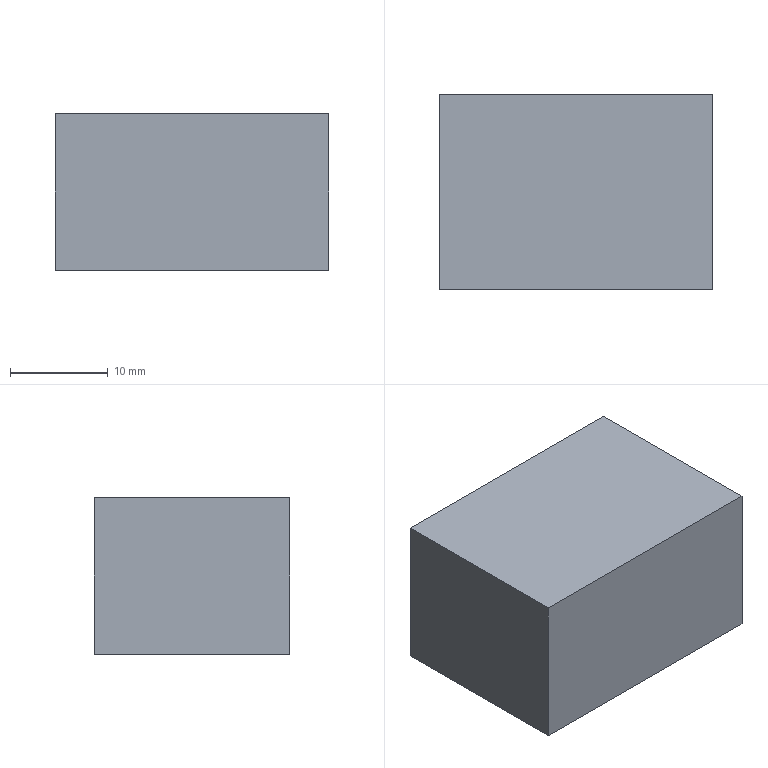Part | SolidWorks | features Extrusion 1 | 1 solid | 6 faces | box 28 x 20 x 16 mm | volume 8960 mm3 | plane 6
STEP:
#1=CARTESIAN_POINT('',(-14.,10.,8.));
#2=VERTEX_POINT('',#1);
#3=CARTESIAN_POINT('',(-14.,-10.,8.));
#4=VERTEX_POINT('',#3);
#5=CARTESIAN_POINT('',(-14.,10.,8.));
#6=DIRECTION('',(0.,-1.,0.));
#7=VECTOR('',#6,1000.);
#8=LINE('',#5,#7);
#9=EDGE_CURVE('',#2,#4,#8,.T.);
#10=ORIENTED_EDGE('',*,*,#9,.F.);
#11=CARTESIAN_POINT('',(-14.,10.,-8.));
#12=VERTEX_POINT('',#11);
#13=CARTESIAN_POINT('',(-14.,10.,-8.));
#14=DIRECTION('',(0.,0.,1.));
#15=VECTOR('',#14,1000.);
#16=LINE('',#13,#15);
#17=EDGE_CURVE('',#12,#2,#16,.T.);
#18=ORIENTED_EDGE('',*,*,#17,.F.);
#19=CARTESIAN_POINT('',(-14.,-10.,-8.));
#20=VERTEX_POINT('',#19);
#21=CARTESIAN_POINT('',(-14.,10.,-8.));
#22=DIRECTION('',(0.,-1.,0.));
#23=VECTOR('',#22,1000.);
#24=LINE('',#21,#23);
#25=EDGE_CURVE('',#12,#20,#24,.T.);
#26=ORIENTED_EDGE('',*,*,#25,.T.);
#27=CARTESIAN_POINT('',(-14.,-10.,-8.));
#28=DIRECTION('',(0.,0.,1.));
#29=VECTOR('',#28,1000.);
#30=LINE('',#27,#29);
#31=EDGE_CURVE('',#20,#4,#30,.T.);
#32=ORIENTED_EDGE('',*,*,#31,.T.);
#33=EDGE_LOOP('',(#10,#18,#26,#32));
#34=FACE_OUTER_BOUND('',#33,.T.);
#35=CARTESIAN_POINT('',(-14.,10.,-8.));
#36=DIRECTION('',(-1.,0.,0.));
#37=DIRECTION('',(0.,0.,1.));
#38=AXIS2_PLACEMENT_3D('',#35,#36,#37);
#39=PLANE('',#38);
#40=ADVANCED_FACE('',(#34),#39,.T.);
#41=CARTESIAN_POINT('',(14.,10.,8.));
#42=VERTEX_POINT('',#41);
#43=CARTESIAN_POINT('',(14.,10.,8.));
#44=DIRECTION('',(-1.,0.,0.));
#45=VECTOR('',#44,1000.);
#46=LINE('',#43,#45);
#47=EDGE_CURVE('',#42,#2,#46,.T.);
#48=ORIENTED_EDGE('',*,*,#47,.F.);
#49=CARTESIAN_POINT('',(14.,10.,-8.));
#50=VERTEX_POINT('',#49);
#51=CARTESIAN_POINT('',(14.,10.,-8.));
#52=DIRECTION('',(0.,0.,1.));
#53=VECTOR('',#52,1000.);
#54=LINE('',#51,#53);
#55=EDGE_CURVE('',#50,#42,#54,.T.);
#56=ORIENTED_EDGE('',*,*,#55,.F.);
#57=CARTESIAN_POINT('',(14.,10.,-8.));
#58=DIRECTION('',(-1.,0.,0.));
#59=VECTOR('',#58,1000.);
#60=LINE('',#57,#59);
#61=EDGE_CURVE('',#50,#12,#60,.T.);
#62=ORIENTED_EDGE('',*,*,#61,.T.);
#63=ORIENTED_EDGE('',*,*,#17,.T.);
#64=EDGE_LOOP('',(#48,#56,#62,#63));
#65=FACE_OUTER_BOUND('',#64,.T.);
#66=CARTESIAN_POINT('',(14.,10.,-8.));
#67=DIRECTION('',(0.,1.,0.));
#68=DIRECTION('',(0.,0.,1.));
#69=AXIS2_PLACEMENT_3D('',#66,#67,#68);
#70=PLANE('',#69);
#71=ADVANCED_FACE('',(#65),#70,.T.);
#72=CARTESIAN_POINT('',(14.,-10.,8.));
#73=VERTEX_POINT('',#72);
#74=CARTESIAN_POINT('',(14.,-10.,8.));
#75=DIRECTION('',(0.,1.,0.));
#76=VECTOR('',#75,1000.);
#77=LINE('',#74,#76);
#78=EDGE_CURVE('',#73,#42,#77,.T.);
#79=ORIENTED_EDGE('',*,*,#78,.F.);
#80=CARTESIAN_POINT('',(14.,-10.,-8.));
#81=VERTEX_POINT('',#80);
#82=CARTESIAN_POINT('',(14.,-10.,-8.));
#83=DIRECTION('',(0.,0.,1.));
#84=VECTOR('',#83,1000.);
#85=LINE('',#82,#84);
#86=EDGE_CURVE('',#81,#73,#85,.T.);
#87=ORIENTED_EDGE('',*,*,#86,.F.);
#88=CARTESIAN_POINT('',(14.,-10.,-8.));
#89=DIRECTION('',(0.,1.,0.));
#90=VECTOR('',#89,1000.);
#91=LINE('',#88,#90);
#92=EDGE_CURVE('',#81,#50,#91,.T.);
#93=ORIENTED_EDGE('',*,*,#92,.T.);
#94=ORIENTED_EDGE('',*,*,#55,.T.);
#95=EDGE_LOOP('',(#79,#87,#93,#94));
#96=FACE_OUTER_BOUND('',#95,.T.);
#97=CARTESIAN_POINT('',(14.,-10.,-8.));
#98=DIRECTION('',(1.,0.,0.));
#99=DIRECTION('',(0.,0.,-1.));
#100=AXIS2_PLACEMENT_3D('',#97,#98,#99);
#101=PLANE('',#100);
#102=ADVANCED_FACE('',(#96),#101,.T.);
#103=CARTESIAN_POINT('',(-14.,-10.,8.));
#104=DIRECTION('',(1.,0.,0.));
#105=VECTOR('',#104,1000.);
#106=LINE('',#103,#105);
#107=EDGE_CURVE('',#4,#73,#106,.T.);
#108=ORIENTED_EDGE('',*,*,#107,.F.);
#109=ORIENTED_EDGE('',*,*,#31,.F.);
#110=CARTESIAN_POINT('',(-14.,-10.,-8.));
#111=DIRECTION('',(1.,0.,0.));
#112=VECTOR('',#111,1000.);
#113=LINE('',#110,#112);
#114=EDGE_CURVE('',#20,#81,#113,.T.);
#115=ORIENTED_EDGE('',*,*,#114,.T.);
#116=ORIENTED_EDGE('',*,*,#86,.T.);
#117=EDGE_LOOP('',(#108,#109,#115,#116));
#118=FACE_OUTER_BOUND('',#117,.T.);
#119=CARTESIAN_POINT('',(-14.,-10.,-8.));
#120=DIRECTION('',(0.,-1.,0.));
#121=DIRECTION('',(0.,0.,-1.));
#122=AXIS2_PLACEMENT_3D('',#119,#120,#121);
#123=PLANE('',#122);
#124=ADVANCED_FACE('',(#118),#123,.T.);
#125=ORIENTED_EDGE('',*,*,#25,.F.);
#126=ORIENTED_EDGE('',*,*,#61,.F.);
#127=ORIENTED_EDGE('',*,*,#92,.F.);
#128=ORIENTED_EDGE('',*,*,#114,.F.);
#129=EDGE_LOOP('',(#125,#126,#127,#128));
#130=FACE_OUTER_BOUND('',#129,.T.);
#131=CARTESIAN_POINT('',(0.,0.,-8.));
#132=DIRECTION('',(0.,0.,1.));
#133=DIRECTION('',(1.,0.,0.));
#134=AXIS2_PLACEMENT_3D('',#131,#132,#133);
#135=PLANE('',#134);
#136=ADVANCED_FACE('',(#130),#135,.F.);
#137=ORIENTED_EDGE('',*,*,#9,.T.);
#138=ORIENTED_EDGE('',*,*,#107,.T.);
#139=ORIENTED_EDGE('',*,*,#78,.T.);
#140=ORIENTED_EDGE('',*,*,#47,.T.);
#141=EDGE_LOOP('',(#137,#138,#139,#140));
#142=FACE_OUTER_BOUND('',#141,.T.);
#143=CARTESIAN_POINT('',(0.,0.,8.));
#144=DIRECTION('',(0.,0.,1.));
#145=DIRECTION('',(1.,0.,0.));
#146=AXIS2_PLACEMENT_3D('',#143,#144,#145);
#147=PLANE('',#146);
#148=ADVANCED_FACE('',(#142),#147,.T.);
#149=CLOSED_SHELL('',(#40,#71,#102,#124,#136,#148));
#150=MANIFOLD_SOLID_BREP('',#149);
#151=CARTESIAN_POINT('',(0.,0.,0.));
#152=DIRECTION('',(0.,0.,1.));
#153=DIRECTION('',(1.,0.,0.));
#154=AXIS2_PLACEMENT_3D('',#151,#152,#153);
#155=(LENGTH_UNIT()NAMED_UNIT(*)SI_UNIT(.MILLI.,.METRE.));
#156=UNCERTAINTY_MEASURE_WITH_UNIT(LENGTH_MEASURE(0.00001),#155,'','');
#157=(NAMED_UNIT(*)PLANE_ANGLE_UNIT()SI_UNIT($,.RADIAN.));
#158=(NAMED_UNIT(*)SI_UNIT($,.STERADIAN.)SOLID_ANGLE_UNIT());
#159=(GEOMETRIC_REPRESENTATION_CONTEXT(3)GLOBAL_UNCERTAINTY_ASSIGNED_CONTEXT((#156))GLOBAL_UNIT_ASSIGNED_CONTEXT((#155,#157,#158))REPRESENTATION_CONTEXT('',''));
#160=ADVANCED_BREP_SHAPE_REPRESENTATION('',(#150,#154),#159);